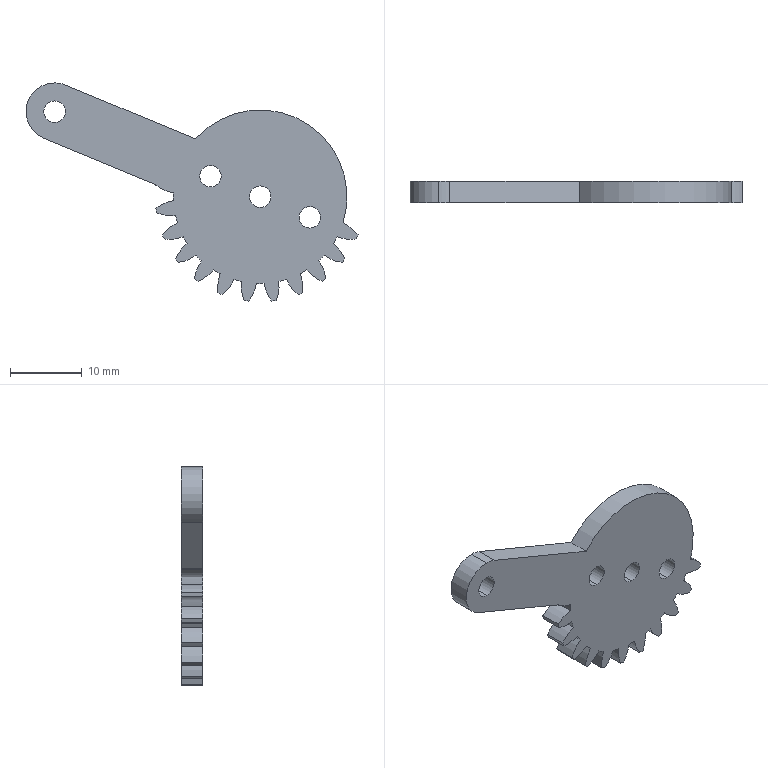Part | SolidWorks | features ICE 2, Extrusion 1 | 1 solid | 66 faces | box 46.268 x 3 x 30.401 mm | volume 1962 mm3 | cylinder 61 | plane 5 | commonest cylinder face diameters 10.8 x26 24.185 x13 29.25 x12 3 x8 8 x2